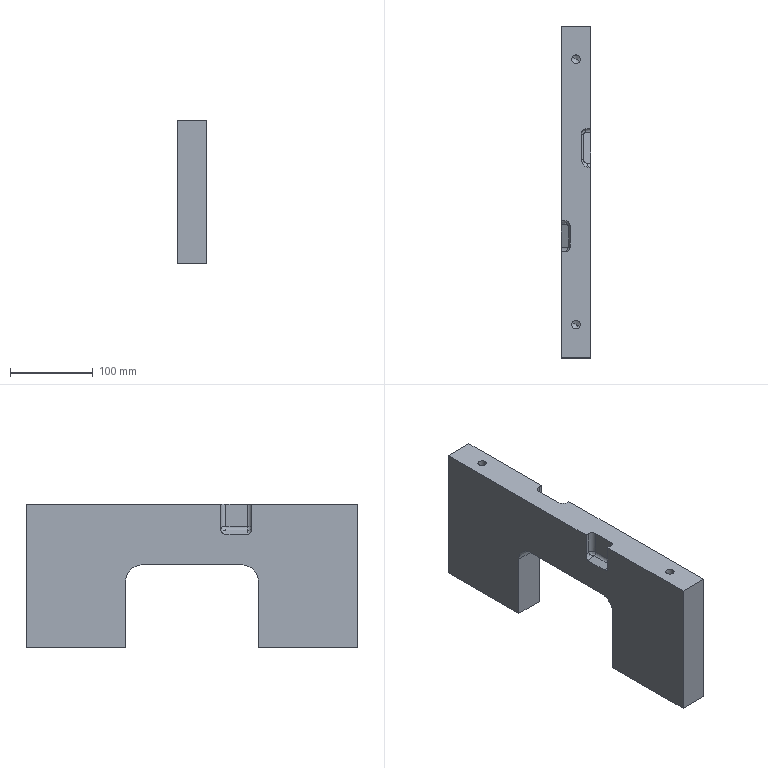Part | CATIA | 1 solid | 50 faces | box 35 x 400 x 173 mm | volume 1827940 mm3 | cylinder 20 | plane 16 | cone 8 | spline 6 | commonest cylinder face diameters 10.2 x8 10 x4 40 x2 11 x1 12.6 x1 14 x1